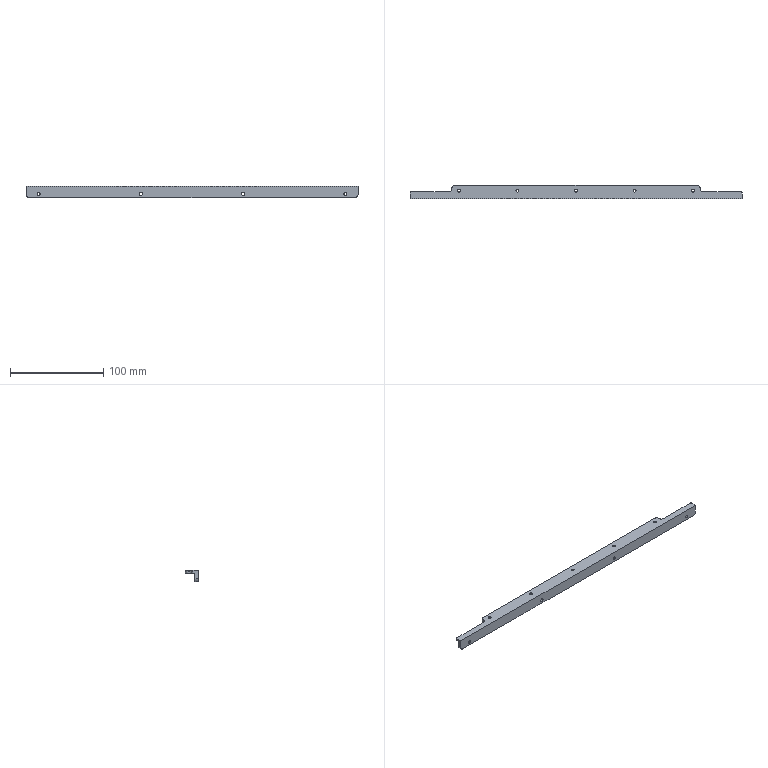NC program | NX | posted with a generic post | part box 356.96 x 14 x 12 mm
Whole program:
N10 G17 G21 G94 G90
(DRILLING_2 , TOOL : D6点钻)
N12 T03 M6
N14 G54
N16 G17 G0 G90 X-165. Y2. B0. C0. S2500 M3
N18 G43 Z50. H3
N20 G94 G81 G98 Z-2. F200. R3.
N22 X-55.
N24 X55.
N26 X165.
N28 G80
N30 G0 X165. Y2. Z50.
N32 M5
(DRILLING_2_COPY , TOOL : Z3.3)
N34 T07 M6
N36 G54
N38 G17 G0 G90 X-165. Y2. B0. C0. S2500 M3
N40 G43 Z50. H7
N42 G94 G81 G98 Z-6. F200. R3.
N44 X-55.
N46 X55.
N48 X165.
N50 G80
N52 G0 X165. Y2. Z50.
N54 M5
(DRILLING_2_COPY_1 , TOOL : M4X0.7)
N56 T08 M6
N58 G54
N60 G17 G0 G90 X-165. Y2. B0. C0. S300 M3
N62 G43 Z50. H8
N64 G84 G94 G98 Z-5. F210. R3.
N66 X-55.
N68 X55.
N70 X165.
N72 G80
N74 G0 X165. Y2. Z50.
N76 M5
N78 M2